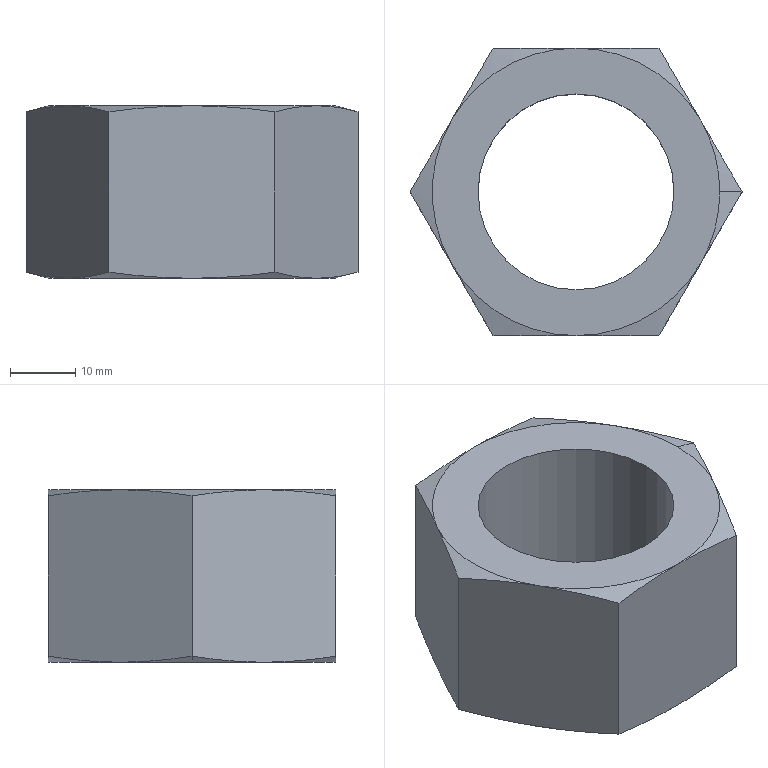Part | SolidWorks | features Cut 2, Chamfer 1, Extrusion 1 | 1 solid | 24 faces | box 50.85 x 44.037 x 26.4 mm | volume 25591 mm3 | cone 14 | plane 8 | cylinder 2 | commonest cylinder face diameters 30 x2
STEP:
#1=CARTESIAN_POINT('',(19.069,11.009,26.4));
#2=VERTEX_POINT('',#1);
#3=CARTESIAN_POINT('',(22.019,0.,26.4));
#4=VERTEX_POINT('',#3);
#5=CARTESIAN_POINT('',(0.,0.,26.4));
#6=DIRECTION('',(0.,0.,-1.));
#7=DIRECTION('',(-1.,0.,0.));
#8=AXIS2_PLACEMENT_3D('',#5,#6,#7);
#9=CIRCLE('',#8,22.019);
#10=EDGE_CURVE('',#2,#4,#9,.T.);
#11=ORIENTED_EDGE('',*,*,#10,.T.);
#12=CARTESIAN_POINT('',(25.425,0.,25.487));
#13=VERTEX_POINT('',#12);
#14=CARTESIAN_POINT('',(22.019,0.,26.4));
#15=DIRECTION('',(0.9659,0.,-0.2588));
#16=VECTOR('',#15,1000.);
#17=LINE('',#14,#16);
#18=EDGE_CURVE('',#4,#13,#17,.T.);
#19=ORIENTED_EDGE('',*,*,#18,.T.);
#20=CARTESIAN_POINT('',(25.425,0.,25.487));
#21=CARTESIAN_POINT('',(24.366,1.835,25.771));
#22=CARTESIAN_POINT('',(23.306,3.67,26.002));
#23=CARTESIAN_POINT('',(21.188,7.34,26.317));
#24=CARTESIAN_POINT('',(20.128,9.174,26.4));
#25=CARTESIAN_POINT('',(19.069,11.009,26.4));
#26=B_SPLINE_CURVE_WITH_KNOTS('',3,(#20,#21,#22,#23,#24,#25),.UNSPECIFIED.,.F.,.F.,(4,2,4),(0.000000231,0.006356,0.01271),.UNSPECIFIED.);
#27=EDGE_CURVE('',#13,#2,#26,.T.);
#28=ORIENTED_EDGE('',*,*,#27,.T.);
#29=EDGE_LOOP('',(#11,#19,#28));
#30=FACE_OUTER_BOUND('',#29,.T.);
#31=CARTESIAN_POINT('',(0.,0.,26.4));
#32=DIRECTION('',(0.,0.,-1.));
#33=DIRECTION('',(1.,0.,0.));
#34=AXIS2_PLACEMENT_3D('',#31,#32,#33);
#35=CONICAL_SURFACE('',#34,22.019,1.309);
#36=ADVANCED_FACE('',(#30),#35,.T.);
#37=CARTESIAN_POINT('',(-22.019,0.,0.));
#38=VERTEX_POINT('',#37);
#39=CARTESIAN_POINT('',(-19.069,11.009,0.));
#40=VERTEX_POINT('',#39);
#41=CARTESIAN_POINT('',(0.,0.,0.));
#42=DIRECTION('',(0.,0.,-1.));
#43=DIRECTION('',(-1.,0.,0.));
#44=AXIS2_PLACEMENT_3D('',#41,#42,#43);
#45=CIRCLE('',#44,22.019);
#46=EDGE_CURVE('',#38,#40,#45,.T.);
#47=ORIENTED_EDGE('',*,*,#46,.F.);
#48=CARTESIAN_POINT('',(-25.425,0.,0.9127));
#49=VERTEX_POINT('',#48);
#50=CARTESIAN_POINT('',(-22.019,0.,0.));
#51=DIRECTION('',(-0.9659,0.,0.2588));
#52=VECTOR('',#51,1000.);
#53=LINE('',#50,#52);
#54=EDGE_CURVE('',#38,#49,#53,.T.);
#55=ORIENTED_EDGE('',*,*,#54,.T.);
#56=CARTESIAN_POINT('',(-25.425,0.,0.9127));
#57=CARTESIAN_POINT('',(-24.366,1.835,0.6289));
#58=CARTESIAN_POINT('',(-23.306,3.67,0.3984));
#59=CARTESIAN_POINT('',(-21.187,7.34,0.08345));
#60=CARTESIAN_POINT('',(-20.128,9.174,0.));
#61=CARTESIAN_POINT('',(-19.069,11.009,0.));
#62=B_SPLINE_CURVE_WITH_KNOTS('',3,(#56,#57,#58,#59,#60,#61),.UNSPECIFIED.,.F.,.F.,(4,2,4),(0.000000231,0.006356,0.01271),.UNSPECIFIED.);
#63=EDGE_CURVE('',#49,#40,#62,.T.);
#64=ORIENTED_EDGE('',*,*,#63,.T.);
#65=EDGE_LOOP('',(#47,#55,#64));
#66=FACE_OUTER_BOUND('',#65,.T.);
#67=CARTESIAN_POINT('',(0.,0.,0.));
#68=DIRECTION('',(0.,0.,1.));
#69=DIRECTION('',(-1.,0.,0.));
#70=AXIS2_PLACEMENT_3D('',#67,#68,#69);
#71=CONICAL_SURFACE('',#70,22.019,1.309);
#72=ADVANCED_FACE('',(#66),#71,.T.);
#73=CARTESIAN_POINT('',(-15.,0.,26.4));
#74=VERTEX_POINT('',#73);
#75=CARTESIAN_POINT('',(15.,0.,26.4));
#76=VERTEX_POINT('',#75);
#77=CARTESIAN_POINT('',(0.,0.,26.4));
#78=DIRECTION('',(0.,0.,1.));
#79=DIRECTION('',(1.,0.,0.));
#80=AXIS2_PLACEMENT_3D('',#77,#78,#79);
#81=CIRCLE('',#80,15.);
#82=EDGE_CURVE('',#74,#76,#81,.T.);
#83=ORIENTED_EDGE('',*,*,#82,.T.);
#84=CARTESIAN_POINT('',(15.,0.,0.));
#85=VERTEX_POINT('',#84);
#86=CARTESIAN_POINT('',(15.,0.,26.4));
#87=DIRECTION('',(0.,0.,-1.));
#88=VECTOR('',#87,1000.);
#89=LINE('',#86,#88);
#90=EDGE_CURVE('',#76,#85,#89,.T.);
#91=ORIENTED_EDGE('',*,*,#90,.T.);
#92=CARTESIAN_POINT('',(-15.,0.,0.));
#93=VERTEX_POINT('',#92);
#94=CARTESIAN_POINT('',(0.,0.,0.));
#95=DIRECTION('',(0.,0.,1.));
#96=DIRECTION('',(1.,0.,0.));
#97=AXIS2_PLACEMENT_3D('',#94,#95,#96);
#98=CIRCLE('',#97,15.);
#99=EDGE_CURVE('',#93,#85,#98,.T.);
#100=ORIENTED_EDGE('',*,*,#99,.F.);
#101=CARTESIAN_POINT('',(-15.,0.,26.4));
#102=DIRECTION('',(0.,0.,-1.));
#103=VECTOR('',#102,1000.);
#104=LINE('',#101,#103);
#105=EDGE_CURVE('',#74,#93,#104,.T.);
#106=ORIENTED_EDGE('',*,*,#105,.F.);
#107=EDGE_LOOP('',(#83,#91,#100,#106));
#108=FACE_OUTER_BOUND('',#107,.T.);
#109=CARTESIAN_POINT('',(0.,0.,26.4));
#110=DIRECTION('',(0.,0.,-1.));
#111=DIRECTION('',(-1.,0.,0.));
#112=AXIS2_PLACEMENT_3D('',#109,#110,#111);
#113=CYLINDRICAL_SURFACE('',#112,15.);
#114=ADVANCED_FACE('',(#108),#113,.F.);
#115=ORIENTED_EDGE('',*,*,#27,.F.);
#116=CARTESIAN_POINT('',(25.425,0.,0.9127));
#117=VERTEX_POINT('',#116);
#118=CARTESIAN_POINT('',(25.425,0.,26.4));
#119=DIRECTION('',(0.,0.,-1.));
#120=VECTOR('',#119,1000.);
#121=LINE('',#118,#120);
#122=EDGE_CURVE('',#13,#117,#121,.T.);
#123=ORIENTED_EDGE('',*,*,#122,.T.);
#124=CARTESIAN_POINT('',(19.069,11.009,0.));
#125=VERTEX_POINT('',#124);
#126=CARTESIAN_POINT('',(19.069,11.009,0.));
#127=CARTESIAN_POINT('',(20.128,9.174,0.));
#128=CARTESIAN_POINT('',(21.188,7.34,0.08345));
#129=CARTESIAN_POINT('',(23.306,3.67,0.3984));
#130=CARTESIAN_POINT('',(24.366,1.835,0.6289));
#131=CARTESIAN_POINT('',(25.425,0.,0.9127));
#132=B_SPLINE_CURVE_WITH_KNOTS('',3,(#126,#127,#128,#129,#130,#131),.UNSPECIFIED.,.F.,.F.,(4,2,4),(0.01271,0.01907,0.02543),.UNSPECIFIED.);
#133=EDGE_CURVE('',#125,#117,#132,.T.);
#134=ORIENTED_EDGE('',*,*,#133,.F.);
#135=CARTESIAN_POINT('',(12.713,22.019,0.9127));
#136=VERTEX_POINT('',#135);
#137=CARTESIAN_POINT('',(12.713,22.019,0.9127));
#138=CARTESIAN_POINT('',(13.772,20.184,0.6289));
#139=CARTESIAN_POINT('',(14.831,18.349,0.3984));
#140=CARTESIAN_POINT('',(16.95,14.679,0.08345));
#141=CARTESIAN_POINT('',(18.009,12.844,0.));
#142=CARTESIAN_POINT('',(19.069,11.009,0.));
#143=B_SPLINE_CURVE_WITH_KNOTS('',3,(#137,#138,#139,#140,#141,#142),.UNSPECIFIED.,.F.,.F.,(4,2,4),(0.000000231,0.006356,0.01271),.UNSPECIFIED.);
#144=EDGE_CURVE('',#136,#125,#143,.T.);
#145=ORIENTED_EDGE('',*,*,#144,.F.);
#146=CARTESIAN_POINT('',(12.713,22.019,25.487));
#147=VERTEX_POINT('',#146);
#148=CARTESIAN_POINT('',(12.713,22.019,26.4));
#149=DIRECTION('',(0.,0.,-1.));
#150=VECTOR('',#149,1000.);
#151=LINE('',#148,#150);
#152=EDGE_CURVE('',#147,#136,#151,.T.);
#153=ORIENTED_EDGE('',*,*,#152,.F.);
#154=CARTESIAN_POINT('',(19.069,11.009,26.4));
#155=CARTESIAN_POINT('',(18.009,12.844,26.4));
#156=CARTESIAN_POINT('',(16.95,14.679,26.317));
#157=CARTESIAN_POINT('',(14.831,18.349,26.002));
#158=CARTESIAN_POINT('',(13.772,20.184,25.771));
#159=CARTESIAN_POINT('',(12.713,22.019,25.487));
#160=B_SPLINE_CURVE_WITH_KNOTS('',3,(#154,#155,#156,#157,#158,#159),.UNSPECIFIED.,.F.,.F.,(4,2,4),(0.01271,0.01907,0.02543),.UNSPECIFIED.);
#161=EDGE_CURVE('',#2,#147,#160,.T.);
#162=ORIENTED_EDGE('',*,*,#161,.F.);
#163=EDGE_LOOP('',(#115,#123,#134,#145,#153,#162));
#164=FACE_OUTER_BOUND('',#163,.T.);
#165=CARTESIAN_POINT('',(25.425,0.,26.4));
#166=DIRECTION('',(-0.866,-0.5,0.));
#167=DIRECTION('',(0.5,-0.866,0.));
#168=AXIS2_PLACEMENT_3D('',#165,#166,#167);
#169=PLANE('',#168);
#170=ADVANCED_FACE('',(#164),#169,.F.);
#171=CARTESIAN_POINT('',(0.,22.019,26.4));
#172=VERTEX_POINT('',#171);
#173=CARTESIAN_POINT('',(12.713,22.019,25.487));
#174=CARTESIAN_POINT('',(10.597,22.019,25.771));
#175=CARTESIAN_POINT('',(8.481,22.019,26.001));
#176=CARTESIAN_POINT('',(4.243,22.019,26.316));
#177=CARTESIAN_POINT('',(2.123,22.019,26.4));
#178=CARTESIAN_POINT('',(0.,22.019,26.4));
#179=B_SPLINE_CURVE_WITH_KNOTS('',3,(#173,#174,#175,#176,#177,#178),.UNSPECIFIED.,.F.,.F.,(4,2,4),(0.06895,0.07535,0.08174),.UNSPECIFIED.);
#180=EDGE_CURVE('',#147,#172,#179,.T.);
#181=ORIENTED_EDGE('',*,*,#180,.F.);
#182=ORIENTED_EDGE('',*,*,#152,.T.);
#183=CARTESIAN_POINT('',(0.,22.019,0.));
#184=VERTEX_POINT('',#183);
#185=CARTESIAN_POINT('',(0.,22.019,0.));
#186=CARTESIAN_POINT('',(2.123,22.019,0.));
#187=CARTESIAN_POINT('',(4.243,22.019,0.08376));
#188=CARTESIAN_POINT('',(8.481,22.019,0.3989));
#189=CARTESIAN_POINT('',(10.597,22.019,0.6293));
#190=CARTESIAN_POINT('',(12.713,22.019,0.9127));
#191=B_SPLINE_CURVE_WITH_KNOTS('',3,(#185,#186,#187,#188,#189,#190),.UNSPECIFIED.,.F.,.F.,(4,2,4),(0.03447,0.04087,0.04728),.UNSPECIFIED.);
#192=EDGE_CURVE('',#184,#136,#191,.T.);
#193=ORIENTED_EDGE('',*,*,#192,.F.);
#194=CARTESIAN_POINT('',(-12.712,22.019,0.9127));
#195=VERTEX_POINT('',#194);
#196=CARTESIAN_POINT('',(-12.712,22.019,0.9127));
#197=CARTESIAN_POINT('',(-10.6,22.019,0.6297));
#198=CARTESIAN_POINT('',(-8.474,22.019,0.3983));
#199=CARTESIAN_POINT('',(-4.234,22.019,0.08324));
#200=CARTESIAN_POINT('',(-2.116,22.019,0.));
#201=CARTESIAN_POINT('',(0.,22.019,0.));
#202=B_SPLINE_CURVE_WITH_KNOTS('',3,(#196,#197,#198,#199,#200,#201),.UNSPECIFIED.,.F.,.F.,(4,2,4),(0.02169,0.02808,0.03447),.UNSPECIFIED.);
#203=EDGE_CURVE('',#195,#184,#202,.T.);
#204=ORIENTED_EDGE('',*,*,#203,.F.);
#205=CARTESIAN_POINT('',(-12.712,22.019,25.487));
#206=VERTEX_POINT('',#205);
#207=CARTESIAN_POINT('',(-12.712,22.019,26.4));
#208=DIRECTION('',(0.,0.,-1.));
#209=VECTOR('',#208,1000.);
#210=LINE('',#207,#209);
#211=EDGE_CURVE('',#206,#195,#210,.T.);
#212=ORIENTED_EDGE('',*,*,#211,.F.);
#213=CARTESIAN_POINT('',(0.,22.019,26.4));
#214=CARTESIAN_POINT('',(-2.116,22.019,26.4));
#215=CARTESIAN_POINT('',(-4.234,22.019,26.317));
#216=CARTESIAN_POINT('',(-8.474,22.019,26.002));
#217=CARTESIAN_POINT('',(-10.6,22.019,25.77));
#218=CARTESIAN_POINT('',(-12.712,22.019,25.487));
#219=B_SPLINE_CURVE_WITH_KNOTS('',3,(#213,#214,#215,#216,#217,#218),.UNSPECIFIED.,.F.,.F.,(4,2,4),(0.08174,0.08811,0.09449),.UNSPECIFIED.);
#220=EDGE_CURVE('',#172,#206,#219,.T.);
#221=ORIENTED_EDGE('',*,*,#220,.F.);
#222=EDGE_LOOP('',(#181,#182,#193,#204,#212,#221));
#223=FACE_OUTER_BOUND('',#222,.T.);
#224=CARTESIAN_POINT('',(12.713,22.019,26.4));
#225=DIRECTION('',(0.,-1.,0.));
#226=DIRECTION('',(1.,0.,0.));
#227=AXIS2_PLACEMENT_3D('',#224,#225,#226);
#228=PLANE('',#227);
#229=ADVANCED_FACE('',(#223),#228,.F.);
#230=CARTESIAN_POINT('',(-19.069,11.009,26.4));
#231=VERTEX_POINT('',#230);
#232=CARTESIAN_POINT('',(-12.712,22.019,25.487));
#233=CARTESIAN_POINT('',(-13.772,20.184,25.771));
#234=CARTESIAN_POINT('',(-14.831,18.349,26.002));
#235=CARTESIAN_POINT('',(-16.95,14.679,26.317));
#236=CARTESIAN_POINT('',(-18.009,12.844,26.4));
#237=CARTESIAN_POINT('',(-19.069,11.009,26.4));
#238=B_SPLINE_CURVE_WITH_KNOTS('',3,(#232,#233,#234,#235,#236,#237),.UNSPECIFIED.,.F.,.F.,(4,2,4),(0.000000231,0.006356,0.01271),.UNSPECIFIED.);
#239=EDGE_CURVE('',#206,#231,#238,.T.);
#240=ORIENTED_EDGE('',*,*,#239,.F.);
#241=ORIENTED_EDGE('',*,*,#211,.T.);
#242=CARTESIAN_POINT('',(-19.069,11.009,0.));
#243=CARTESIAN_POINT('',(-18.009,12.844,0.));
#244=CARTESIAN_POINT('',(-16.95,14.679,0.08345));
#245=CARTESIAN_POINT('',(-14.831,18.349,0.3984));
#246=CARTESIAN_POINT('',(-13.772,20.184,0.6289));
#247=CARTESIAN_POINT('',(-12.712,22.019,0.9127));
#248=B_SPLINE_CURVE_WITH_KNOTS('',3,(#242,#243,#244,#245,#246,#247),.UNSPECIFIED.,.F.,.F.,(4,2,4),(0.01271,0.01907,0.02543),.UNSPECIFIED.);
#249=EDGE_CURVE('',#40,#195,#248,.T.);
#250=ORIENTED_EDGE('',*,*,#249,.F.);
#251=ORIENTED_EDGE('',*,*,#63,.F.);
#252=CARTESIAN_POINT('',(-25.425,0.,25.487));
#253=VERTEX_POINT('',#252);
#254=CARTESIAN_POINT('',(-25.425,0.,26.4));
#255=DIRECTION('',(0.,0.,-1.));
#256=VECTOR('',#255,1000.);
#257=LINE('',#254,#256);
#258=EDGE_CURVE('',#253,#49,#257,.T.);
#259=ORIENTED_EDGE('',*,*,#258,.F.);
#260=CARTESIAN_POINT('',(-19.069,11.009,26.4));
#261=CARTESIAN_POINT('',(-20.128,9.174,26.4));
#262=CARTESIAN_POINT('',(-21.187,7.34,26.317));
#263=CARTESIAN_POINT('',(-23.306,3.67,26.002));
#264=CARTESIAN_POINT('',(-24.366,1.835,25.771));
#265=CARTESIAN_POINT('',(-25.425,0.,25.487));
#266=B_SPLINE_CURVE_WITH_KNOTS('',3,(#260,#261,#262,#263,#264,#265),.UNSPECIFIED.,.F.,.F.,(4,2,4),(0.01271,0.01907,0.02543),.UNSPECIFIED.);
#267=EDGE_CURVE('',#231,#253,#266,.T.);
#268=ORIENTED_EDGE('',*,*,#267,.F.);
#269=EDGE_LOOP('',(#240,#241,#250,#251,#259,#268));
#270=FACE_OUTER_BOUND('',#269,.T.);
#271=CARTESIAN_POINT('',(-12.712,22.019,26.4));
#272=DIRECTION('',(0.866,-0.5,0.));
#273=DIRECTION('',(0.5,0.866,0.));
#274=AXIS2_PLACEMENT_3D('',#271,#272,#273);
#275=PLANE('',#274);
#276=ADVANCED_FACE('',(#270),#275,.F.);
#277=CARTESIAN_POINT('',(-19.069,-11.009,26.4));
#278=VERTEX_POINT('',#277);
#279=CARTESIAN_POINT('',(-25.425,0.,25.487));
#280=CARTESIAN_POINT('',(-24.366,-1.835,25.771));
#281=CARTESIAN_POINT('',(-23.306,-3.67,26.002));
#282=CARTESIAN_POINT('',(-21.187,-7.34,26.317));
#283=CARTESIAN_POINT('',(-20.128,-9.174,26.4));
#284=CARTESIAN_POINT('',(-19.069,-11.009,26.4));
#285=B_SPLINE_CURVE_WITH_KNOTS('',3,(#279,#280,#281,#282,#283,#284),.UNSPECIFIED.,.F.,.F.,(4,2,4),(0.000000231,0.006356,0.01271),.UNSPECIFIED.);
#286=EDGE_CURVE('',#253,#278,#285,.T.);
#287=ORIENTED_EDGE('',*,*,#286,.F.);
#288=ORIENTED_EDGE('',*,*,#258,.T.);
#289=CARTESIAN_POINT('',(-19.069,-11.009,0.));
#290=VERTEX_POINT('',#289);
#291=CARTESIAN_POINT('',(-19.069,-11.009,0.));
#292=CARTESIAN_POINT('',(-20.128,-9.174,0.));
#293=CARTESIAN_POINT('',(-21.188,-7.34,0.08345));
#294=CARTESIAN_POINT('',(-23.306,-3.67,0.3984));
#295=CARTESIAN_POINT('',(-24.366,-1.835,0.6289));
#296=CARTESIAN_POINT('',(-25.425,0.,0.9127));
#297=B_SPLINE_CURVE_WITH_KNOTS('',3,(#291,#292,#293,#294,#295,#296),.UNSPECIFIED.,.F.,.F.,(4,2,4),(0.01271,0.01907,0.02543),.UNSPECIFIED.);
#298=EDGE_CURVE('',#290,#49,#297,.T.);
#299=ORIENTED_EDGE('',*,*,#298,.F.);
#300=CARTESIAN_POINT('',(-12.713,-22.019,0.9127));
#301=VERTEX_POINT('',#300);
#302=CARTESIAN_POINT('',(-12.713,-22.019,0.9127));
#303=CARTESIAN_POINT('',(-13.772,-20.184,0.6289));
#304=CARTESIAN_POINT('',(-14.831,-18.349,0.3984));
#305=CARTESIAN_POINT('',(-16.95,-14.679,0.08345));
#306=CARTESIAN_POINT('',(-18.009,-12.844,0.));
#307=CARTESIAN_POINT('',(-19.069,-11.009,0.));
#308=B_SPLINE_CURVE_WITH_KNOTS('',3,(#302,#303,#304,#305,#306,#307),.UNSPECIFIED.,.F.,.F.,(4,2,4),(0.000000231,0.006356,0.01271),.UNSPECIFIED.);
#309=EDGE_CURVE('',#301,#290,#308,.T.);
#310=ORIENTED_EDGE('',*,*,#309,.F.);
#311=CARTESIAN_POINT('',(-12.713,-22.019,25.487));
#312=VERTEX_POINT('',#311);
#313=CARTESIAN_POINT('',(-12.712,-22.019,26.4));
#314=DIRECTION('',(0.,0.,-1.));
#315=VECTOR('',#314,1000.);
#316=LINE('',#313,#315);
#317=EDGE_CURVE('',#312,#301,#316,.T.);
#318=ORIENTED_EDGE('',*,*,#317,.F.);
#319=CARTESIAN_POINT('',(-19.069,-11.009,26.4));
#320=CARTESIAN_POINT('',(-18.009,-12.844,26.4));
#321=CARTESIAN_POINT('',(-16.95,-14.679,26.317));
#322=CARTESIAN_POINT('',(-14.831,-18.349,26.002));
#323=CARTESIAN_POINT('',(-13.772,-20.184,25.771));
#324=CARTESIAN_POINT('',(-12.713,-22.019,25.487));
#325=B_SPLINE_CURVE_WITH_KNOTS('',3,(#319,#320,#321,#322,#323,#324),.UNSPECIFIED.,.F.,.F.,(4,2,4),(0.01271,0.01907,0.02543),.UNSPECIFIED.);
#326=EDGE_CURVE('',#278,#312,#325,.T.);
#327=ORIENTED_EDGE('',*,*,#326,.F.);
#328=EDGE_LOOP('',(#287,#288,#299,#310,#318,#327));
#329=FACE_OUTER_BOUND('',#328,.T.);
#330=CARTESIAN_POINT('',(-25.425,0.,26.4));
#331=DIRECTION('',(0.866,0.5,0.));
#332=DIRECTION('',(-0.5,0.866,0.));
#333=AXIS2_PLACEMENT_3D('',#330,#331,#332);
#334=PLANE('',#333);
#335=ADVANCED_FACE('',(#329),#334,.F.);
#336=CARTESIAN_POINT('',(0.,-22.019,26.4));
#337=VERTEX_POINT('',#336);
#338=CARTESIAN_POINT('',(-12.713,-22.019,25.487));
#339=CARTESIAN_POINT('',(-10.6,-22.019,25.77));
#340=CARTESIAN_POINT('',(-8.474,-22.019,26.002));
#341=CARTESIAN_POINT('',(-4.234,-22.019,26.317));
#342=CARTESIAN_POINT('',(-2.116,-22.019,26.4));
#343=CARTESIAN_POINT('',(0.,-22.019,26.4));
#344=B_SPLINE_CURVE_WITH_KNOTS('',3,(#338,#339,#340,#341,#342,#343),.UNSPECIFIED.,.F.,.F.,(4,2,4),(0.02169,0.02808,0.03447),.UNSPECIFIED.);
#345=EDGE_CURVE('',#312,#337,#344,.T.);
#346=ORIENTED_EDGE('',*,*,#345,.F.);
#347=ORIENTED_EDGE('',*,*,#317,.T.);
#348=CARTESIAN_POINT('',(0.,-22.019,0.));
#349=VERTEX_POINT('',#348);
#350=CARTESIAN_POINT('',(0.,-22.019,0.));
#351=CARTESIAN_POINT('',(-2.116,-22.019,0.));
#352=CARTESIAN_POINT('',(-4.234,-22.019,0.08324));
#353=CARTESIAN_POINT('',(-8.474,-22.019,0.3983));
#354=CARTESIAN_POINT('',(-10.6,-22.019,0.6297));
#355=CARTESIAN_POINT('',(-12.713,-22.019,0.9127));
#356=B_SPLINE_CURVE_WITH_KNOTS('',3,(#350,#351,#352,#353,#354,#355),.UNSPECIFIED.,.F.,.F.,(4,2,4),(0.08174,0.08811,0.09449),.UNSPECIFIED.);
#357=EDGE_CURVE('',#349,#301,#356,.T.);
#358=ORIENTED_EDGE('',*,*,#357,.F.);
#359=CARTESIAN_POINT('',(12.713,-22.019,0.9127));
#360=VERTEX_POINT('',#359);
#361=CARTESIAN_POINT('',(12.713,-22.019,0.9127));
#362=CARTESIAN_POINT('',(10.597,-22.019,0.6293));
#363=CARTESIAN_POINT('',(8.481,-22.019,0.3989));
#364=CARTESIAN_POINT('',(4.243,-22.019,0.08376));
#365=CARTESIAN_POINT('',(2.123,-22.019,0.));
#366=CARTESIAN_POINT('',(0.,-22.019,0.));
#367=B_SPLINE_CURVE_WITH_KNOTS('',3,(#361,#362,#363,#364,#365,#366),.UNSPECIFIED.,.F.,.F.,(4,2,4),(0.06895,0.07535,0.08174),.UNSPECIFIED.);
#368=EDGE_CURVE('',#360,#349,#367,.T.);
#369=ORIENTED_EDGE('',*,*,#368,.F.);
#370=CARTESIAN_POINT('',(12.713,-22.019,25.487));
#371=VERTEX_POINT('',#370);
#372=CARTESIAN_POINT('',(12.713,-22.019,26.4));
#373=DIRECTION('',(0.,0.,-1.));
#374=VECTOR('',#373,1000.);
#375=LINE('',#372,#374);
#376=EDGE_CURVE('',#371,#360,#375,.T.);
#377=ORIENTED_EDGE('',*,*,#376,.F.);
#378=CARTESIAN_POINT('',(0.,-22.019,26.4));
#379=CARTESIAN_POINT('',(2.123,-22.019,26.4));
#380=CARTESIAN_POINT('',(4.243,-22.019,26.316));
#381=CARTESIAN_POINT('',(8.481,-22.019,26.001));
#382=CARTESIAN_POINT('',(10.597,-22.019,25.771));
#383=CARTESIAN_POINT('',(12.713,-22.019,25.487));
#384=B_SPLINE_CURVE_WITH_KNOTS('',3,(#378,#379,#380,#381,#382,#383),.UNSPECIFIED.,.F.,.F.,(4,2,4),(0.03447,0.04087,0.04728),.UNSPECIFIED.);
#385=EDGE_CURVE('',#337,#371,#384,.T.);
#386=ORIENTED_EDGE('',*,*,#385,.F.);
#387=EDGE_LOOP('',(#346,#347,#358,#369,#377,#386));
#388=FACE_OUTER_BOUND('',#387,.T.);
#389=CARTESIAN_POINT('',(-12.712,-22.019,26.4));
#390=DIRECTION('',(0.,1.,0.));
#391=DIRECTION('',(-1.,0.,0.));
#392=AXIS2_PLACEMENT_3D('',#389,#390,#391);
#393=PLANE('',#392);
#394=ADVANCED_FACE('',(#388),#393,.F.);
#395=CARTESIAN_POINT('',(19.069,-11.009,26.4));
#396=VERTEX_POINT('',#395);
#397=CARTESIAN_POINT('',(12.713,-22.019,25.487));
#398=CARTESIAN_POINT('',(13.772,-20.184,25.771));
#399=CARTESIAN_POINT('',(14.831,-18.349,26.002));
#400=CARTESIAN_POINT('',(16.95,-14.679,26.317));
#401=CARTESIAN_POINT('',(18.009,-12.844,26.4));
#402=CARTESIAN_POINT('',(19.069,-11.009,26.4));
#403=B_SPLINE_CURVE_WITH_KNOTS('',3,(#397,#398,#399,#400,#401,#402),.UNSPECIFIED.,.F.,.F.,(4,2,4),(0.000000231,0.006356,0.01271),.UNSPECIFIED.);
#404=EDGE_CURVE('',#371,#396,#403,.T.);
#405=ORIENTED_EDGE('',*,*,#404,.F.);
#406=ORIENTED_EDGE('',*,*,#376,.T.);
#407=CARTESIAN_POINT('',(19.069,-11.009,0.));
#408=VERTEX_POINT('',#407);
#409=CARTESIAN_POINT('',(19.069,-11.009,0.));
#410=CARTESIAN_POINT('',(18.009,-12.844,0.));
#411=CARTESIAN_POINT('',(16.95,-14.679,0.08345));
#412=CARTESIAN_POINT('',(14.831,-18.349,0.3984));
#413=CARTESIAN_POINT('',(13.772,-20.184,0.6289));
#414=CARTESIAN_POINT('',(12.713,-22.019,0.9127));
#415=B_SPLINE_CURVE_WITH_KNOTS('',3,(#409,#410,#411,#412,#413,#414),.UNSPECIFIED.,.F.,.F.,(4,2,4),(0.01271,0.01907,0.02543),.UNSPECIFIED.);
#416=EDGE_CURVE('',#408,#360,#415,.T.);
#417=ORIENTED_EDGE('',*,*,#416,.F.);
#418=CARTESIAN_POINT('',(25.425,0.,0.9127));
#419=CARTESIAN_POINT('',(24.366,-1.835,0.6289));
#420=CARTESIAN_POINT('',(23.306,-3.67,0.3984));
#421=CARTESIAN_POINT('',(21.188,-7.34,0.08345));
#422=CARTESIAN_POINT('',(20.128,-9.174,0.));
#423=CARTESIAN_POINT('',(19.069,-11.009,0.));
#424=B_SPLINE_CURVE_WITH_KNOTS('',3,(#418,#419,#420,#421,#422,#423),.UNSPECIFIED.,.F.,.F.,(4,2,4),(0.000000231,0.006356,0.01271),.UNSPECIFIED.);
#425=EDGE_CURVE('',#117,#408,#424,.T.);
#426=ORIENTED_EDGE('',*,*,#425,.F.);
#427=ORIENTED_EDGE('',*,*,#122,.F.);
#428=CARTESIAN_POINT('',(19.069,-11.009,26.4));
#429=CARTESIAN_POINT('',(20.128,-9.174,26.4));
#430=CARTESIAN_POINT('',(21.188,-7.34,26.317));
#431=CARTESIAN_POINT('',(23.306,-3.67,26.002));
#432=CARTESIAN_POINT('',(24.366,-1.835,25.771));
#433=CARTESIAN_POINT('',(25.425,0.,25.487));
#434=B_SPLINE_CURVE_WITH_KNOTS('',3,(#428,#429,#430,#431,#432,#433),.UNSPECIFIED.,.F.,.F.,(4,2,4),(0.01271,0.01907,0.02543),.UNSPECIFIED.);
#435=EDGE_CURVE('',#396,#13,#434,.T.);
#436=ORIENTED_EDGE('',*,*,#435,.F.);
#437=EDGE_LOOP('',(#405,#406,#417,#426,#427,#436));
#438=FACE_OUTER_BOUND('',#437,.T.);
#439=CARTESIAN_POINT('',(12.713,-22.019,26.4));
#440=DIRECTION('',(-0.866,0.5,0.));
#441=DIRECTION('',(-0.5,-0.866,0.));
#442=AXIS2_PLACEMENT_3D('',#439,#440,#441);
#443=PLANE('',#442);
#444=ADVANCED_FACE('',(#438),#443,.F.);
#445=ORIENTED_EDGE('',*,*,#82,.F.);
#446=CARTESIAN_POINT('',(0.,0.,26.4));
#447=DIRECTION('',(0.,0.,1.));
#448=DIRECTION('',(1.,0.,0.));
#449=AXIS2_PLACEMENT_3D('',#446,#447,#448);
#450=CIRCLE('',#449,15.);
#451=EDGE_CURVE('',#76,#74,#450,.T.);
#452=ORIENTED_EDGE('',*,*,#451,.F.);
#453=EDGE_LOOP('',(#445,#452));
#454=FACE_BOUND('',#453,.T.);
#455=CARTESIAN_POINT('',(0.,0.,26.4));
#456=DIRECTION('',(0.,0.,-1.));
#457=DIRECTION('',(-1.,0.,0.));
#458=AXIS2_PLACEMENT_3D('',#455,#456,#457);
#459=CIRCLE('',#458,22.019);
#460=EDGE_CURVE('',#231,#172,#459,.T.);
#461=ORIENTED_EDGE('',*,*,#460,.F.);
#462=CARTESIAN_POINT('',(0.,0.,26.4));
#463=DIRECTION('',(0.,0.,-1.));
#464=DIRECTION('',(-1.,0.,0.));
#465=AXIS2_PLACEMENT_3D('',#462,#463,#464);
#466=CIRCLE('',#465,22.019);
#467=EDGE_CURVE('',#278,#231,#466,.T.);
#468=ORIENTED_EDGE('',*,*,#467,.F.);
#469=CARTESIAN_POINT('',(0.,0.,26.4));
#470=DIRECTION('',(0.,0.,-1.));
#471=DIRECTION('',(-1.,0.,0.));
#472=AXIS2_PLACEMENT_3D('',#469,#470,#471);
#473=CIRCLE('',#472,22.019);
#474=EDGE_CURVE('',#337,#278,#473,.T.);
#475=ORIENTED_EDGE('',*,*,#474,.F.);
#476=CARTESIAN_POINT('',(0.,0.,26.4));
#477=DIRECTION('',(0.,0.,-1.));
#478=DIRECTION('',(-1.,0.,0.));
#479=AXIS2_PLACEMENT_3D('',#476,#477,#478);
#480=CIRCLE('',#479,22.019);
#481=EDGE_CURVE('',#396,#337,#480,.T.);
#482=ORIENTED_EDGE('',*,*,#481,.F.);
#483=CARTESIAN_POINT('',(0.,0.,26.4));
#484=DIRECTION('',(0.,0.,-1.));
#485=DIRECTION('',(-1.,0.,0.));
#486=AXIS2_PLACEMENT_3D('',#483,#484,#485);
#487=CIRCLE('',#486,22.019);
#488=EDGE_CURVE('',#4,#396,#487,.T.);
#489=ORIENTED_EDGE('',*,*,#488,.F.);
#490=ORIENTED_EDGE('',*,*,#10,.F.);
#491=CARTESIAN_POINT('',(0.,0.,26.4));
#492=DIRECTION('',(0.,0.,1.));
#493=DIRECTION('',(1.,0.,0.));
#494=AXIS2_PLACEMENT_3D('',#491,#492,#493);
#495=CIRCLE('',#494,22.019);
#496=EDGE_CURVE('',#2,#172,#495,.T.);
#497=ORIENTED_EDGE('',*,*,#496,.T.);
#498=EDGE_LOOP('',(#461,#468,#475,#482,#489,#490,#497));
#499=FACE_OUTER_BOUND('',#498,.T.);
#500=CARTESIAN_POINT('',(38.137,-22.019,26.4));
#501=DIRECTION('',(0.,0.,-1.));
#502=DIRECTION('',(-1.,0.,0.));
#503=AXIS2_PLACEMENT_3D('',#500,#501,#502);
#504=PLANE('',#503);
#505=ADVANCED_FACE('',(#454,#499),#504,.F.);
#506=ORIENTED_EDGE('',*,*,#99,.T.);
#507=CARTESIAN_POINT('',(0.,0.,0.));
#508=DIRECTION('',(0.,0.,1.));
#509=DIRECTION('',(1.,0.,0.));
#510=AXIS2_PLACEMENT_3D('',#507,#508,#509);
#511=CIRCLE('',#510,15.);
#512=EDGE_CURVE('',#85,#93,#511,.T.);
#513=ORIENTED_EDGE('',*,*,#512,.T.);
#514=EDGE_LOOP('',(#506,#513));
#515=FACE_BOUND('',#514,.T.);
#516=CARTESIAN_POINT('',(0.,0.,0.));
#517=DIRECTION('',(0.,0.,-1.));
#518=DIRECTION('',(-1.,0.,0.));
#519=AXIS2_PLACEMENT_3D('',#516,#517,#518);
#520=CIRCLE('',#519,22.019);
#521=EDGE_CURVE('',#290,#38,#520,.T.);
#522=ORIENTED_EDGE('',*,*,#521,.T.);
#523=ORIENTED_EDGE('',*,*,#46,.T.);
#524=CARTESIAN_POINT('',(0.,0.,0.));
#525=DIRECTION('',(0.,0.,-1.));
#526=DIRECTION('',(-1.,0.,0.));
#527=AXIS2_PLACEMENT_3D('',#524,#525,#526);
#528=CIRCLE('',#527,22.019);
#529=EDGE_CURVE('',#40,#184,#528,.T.);
#530=ORIENTED_EDGE('',*,*,#529,.T.);
#531=CARTESIAN_POINT('',(0.,0.,0.));
#532=DIRECTION('',(0.,0.,-1.));
#533=DIRECTION('',(-1.,0.,0.));
#534=AXIS2_PLACEMENT_3D('',#531,#532,#533);
#535=CIRCLE('',#534,22.019);
#536=EDGE_CURVE('',#184,#125,#535,.T.);
#537=ORIENTED_EDGE('',*,*,#536,.T.);
#538=CARTESIAN_POINT('',(0.,0.,0.));
#539=DIRECTION('',(0.,0.,-1.));
#540=DIRECTION('',(-1.,0.,0.));
#541=AXIS2_PLACEMENT_3D('',#538,#539,#540);
#542=CIRCLE('',#541,22.019);
#543=EDGE_CURVE('',#125,#408,#542,.T.);
#544=ORIENTED_EDGE('',*,*,#543,.T.);
#545=CARTESIAN_POINT('',(0.,0.,0.));
#546=DIRECTION('',(0.,0.,-1.));
#547=DIRECTION('',(-1.,0.,0.));
#548=AXIS2_PLACEMENT_3D('',#545,#546,#547);
#549=CIRCLE('',#548,22.019);
#550=EDGE_CURVE('',#408,#349,#549,.T.);
#551=ORIENTED_EDGE('',*,*,#550,.T.);
#552=CARTESIAN_POINT('',(0.,0.,0.));
#553=DIRECTION('',(0.,0.,-1.));
#554=DIRECTION('',(-1.,0.,0.));
#555=AXIS2_PLACEMENT_3D('',#552,#553,#554);
#556=CIRCLE('',#555,22.019);
#557=EDGE_CURVE('',#349,#290,#556,.T.);
#558=ORIENTED_EDGE('',*,*,#557,.T.);
#559=EDGE_LOOP('',(#522,#523,#530,#537,#544,#551,#558));
#560=FACE_OUTER_BOUND('',#559,.T.);
#561=CARTESIAN_POINT('',(38.137,-22.019,0.));
#562=DIRECTION('',(0.,0.,-1.));
#563=DIRECTION('',(-1.,0.,0.));
#564=AXIS2_PLACEMENT_3D('',#561,#562,#563);
#565=PLANE('',#564);
#566=ADVANCED_FACE('',(#515,#560),#565,.T.);
#567=ORIENTED_EDGE('',*,*,#90,.F.);
#568=ORIENTED_EDGE('',*,*,#451,.T.);
#569=ORIENTED_EDGE('',*,*,#105,.T.);
#570=ORIENTED_EDGE('',*,*,#512,.F.);
#571=EDGE_LOOP('',(#567,#568,#569,#570));
#572=FACE_OUTER_BOUND('',#571,.T.);
#573=CARTESIAN_POINT('',(0.,0.,26.4));
#574=DIRECTION('',(0.,0.,-1.));
#575=DIRECTION('',(-1.,0.,0.));
#576=AXIS2_PLACEMENT_3D('',#573,#574,#575);
#577=CYLINDRICAL_SURFACE('',#576,15.);
#578=ADVANCED_FACE('',(#572),#577,.F.);
#579=ORIENTED_EDGE('',*,*,#368,.T.);
#580=ORIENTED_EDGE('',*,*,#550,.F.);
#581=ORIENTED_EDGE('',*,*,#416,.T.);
#582=EDGE_LOOP('',(#579,#580,#581));
#583=FACE_OUTER_BOUND('',#582,.T.);
#584=CARTESIAN_POINT('',(0.,0.,0.));
#585=DIRECTION('',(0.,0.,1.));
#586=DIRECTION('',(-1.,0.,0.));
#587=AXIS2_PLACEMENT_3D('',#584,#585,#586);
#588=CONICAL_SURFACE('',#587,22.019,1.309);
#589=ADVANCED_FACE('',(#583),#588,.T.);
#590=ORIENTED_EDGE('',*,*,#133,.T.);
#591=ORIENTED_EDGE('',*,*,#425,.T.);
#592=ORIENTED_EDGE('',*,*,#543,.F.);
#593=EDGE_LOOP('',(#590,#591,#592));
#594=FACE_OUTER_BOUND('',#593,.T.);
#595=CARTESIAN_POINT('',(0.,0.,0.));
#596=DIRECTION('',(0.,0.,1.));
#597=DIRECTION('',(-1.,0.,0.));
#598=AXIS2_PLACEMENT_3D('',#595,#596,#597);
#599=CONICAL_SURFACE('',#598,22.019,1.309);
#600=ADVANCED_FACE('',(#594),#599,.T.);
#601=ORIENTED_EDGE('',*,*,#309,.T.);
#602=ORIENTED_EDGE('',*,*,#557,.F.);
#603=ORIENTED_EDGE('',*,*,#357,.T.);
#604=EDGE_LOOP('',(#601,#602,#603));
#605=FACE_OUTER_BOUND('',#604,.T.);
#606=CARTESIAN_POINT('',(0.,0.,0.));
#607=DIRECTION('',(0.,0.,1.));
#608=DIRECTION('',(-1.,0.,0.));
#609=AXIS2_PLACEMENT_3D('',#606,#607,#608);
#610=CONICAL_SURFACE('',#609,22.019,1.309);
#611=ADVANCED_FACE('',(#605),#610,.T.);
#612=ORIENTED_EDGE('',*,*,#54,.F.);
#613=ORIENTED_EDGE('',*,*,#521,.F.);
#614=ORIENTED_EDGE('',*,*,#298,.T.);
#615=EDGE_LOOP('',(#612,#613,#614));
#616=FACE_OUTER_BOUND('',#615,.T.);
#617=CARTESIAN_POINT('',(0.,0.,0.));
#618=DIRECTION('',(0.,0.,1.));
#619=DIRECTION('',(-1.,0.,0.));
#620=AXIS2_PLACEMENT_3D('',#617,#618,#619);
#621=CONICAL_SURFACE('',#620,22.019,1.309);
#622=ADVANCED_FACE('',(#616),#621,.T.);
#623=ORIENTED_EDGE('',*,*,#249,.T.);
#624=ORIENTED_EDGE('',*,*,#203,.T.);
#625=ORIENTED_EDGE('',*,*,#529,.F.);
#626=EDGE_LOOP('',(#623,#624,#625));
#627=FACE_OUTER_BOUND('',#626,.T.);
#628=CARTESIAN_POINT('',(0.,0.,0.));
#629=DIRECTION('',(0.,0.,1.));
#630=DIRECTION('',(-1.,0.,0.));
#631=AXIS2_PLACEMENT_3D('',#628,#629,#630);
#632=CONICAL_SURFACE('',#631,22.019,1.309);
#633=ADVANCED_FACE('',(#627),#632,.T.);
#634=ORIENTED_EDGE('',*,*,#192,.T.);
#635=ORIENTED_EDGE('',*,*,#144,.T.);
#636=ORIENTED_EDGE('',*,*,#536,.F.);
#637=EDGE_LOOP('',(#634,#635,#636));
#638=FACE_OUTER_BOUND('',#637,.T.);
#639=CARTESIAN_POINT('',(0.,0.,0.));
#640=DIRECTION('',(0.,0.,1.));
#641=DIRECTION('',(-1.,0.,0.));
#642=AXIS2_PLACEMENT_3D('',#639,#640,#641);
#643=CONICAL_SURFACE('',#642,22.019,1.309);
#644=ADVANCED_FACE('',(#638),#643,.T.);
#645=ORIENTED_EDGE('',*,*,#267,.T.);
#646=ORIENTED_EDGE('',*,*,#286,.T.);
#647=ORIENTED_EDGE('',*,*,#467,.T.);
#648=EDGE_LOOP('',(#645,#646,#647));
#649=FACE_OUTER_BOUND('',#648,.T.);
#650=CARTESIAN_POINT('',(0.,0.,26.4));
#651=DIRECTION('',(0.,0.,-1.));
#652=DIRECTION('',(1.,0.,0.));
#653=AXIS2_PLACEMENT_3D('',#650,#651,#652);
#654=CONICAL_SURFACE('',#653,22.019,1.309);
#655=ADVANCED_FACE('',(#649),#654,.T.);
#656=ORIENTED_EDGE('',*,*,#326,.T.);
#657=ORIENTED_EDGE('',*,*,#345,.T.);
#658=ORIENTED_EDGE('',*,*,#474,.T.);
#659=EDGE_LOOP('',(#656,#657,#658));
#660=FACE_OUTER_BOUND('',#659,.T.);
#661=CARTESIAN_POINT('',(0.,0.,26.4));
#662=DIRECTION('',(0.,0.,-1.));
#663=DIRECTION('',(1.,0.,0.));
#664=AXIS2_PLACEMENT_3D('',#661,#662,#663);
#665=CONICAL_SURFACE('',#664,22.019,1.309);
#666=ADVANCED_FACE('',(#660),#665,.T.);
#667=ORIENTED_EDGE('',*,*,#385,.T.);
#668=ORIENTED_EDGE('',*,*,#404,.T.);
#669=ORIENTED_EDGE('',*,*,#481,.T.);
#670=EDGE_LOOP('',(#667,#668,#669));
#671=FACE_OUTER_BOUND('',#670,.T.);
#672=CARTESIAN_POINT('',(0.,0.,26.4));
#673=DIRECTION('',(0.,0.,-1.));
#674=DIRECTION('',(1.,0.,0.));
#675=AXIS2_PLACEMENT_3D('',#672,#673,#674);
#676=CONICAL_SURFACE('',#675,22.019,1.309);
#677=ADVANCED_FACE('',(#671),#676,.T.);
#678=ORIENTED_EDGE('',*,*,#18,.F.);
#679=ORIENTED_EDGE('',*,*,#488,.T.);
#680=ORIENTED_EDGE('',*,*,#435,.T.);
#681=EDGE_LOOP('',(#678,#679,#680));
#682=FACE_OUTER_BOUND('',#681,.T.);
#683=CARTESIAN_POINT('',(0.,0.,26.4));
#684=DIRECTION('',(0.,0.,-1.));
#685=DIRECTION('',(1.,0.,0.));
#686=AXIS2_PLACEMENT_3D('',#683,#684,#685);
#687=CONICAL_SURFACE('',#686,22.019,1.309);
#688=ADVANCED_FACE('',(#682),#687,.T.);
#689=ORIENTED_EDGE('',*,*,#161,.T.);
#690=ORIENTED_EDGE('',*,*,#180,.T.);
#691=ORIENTED_EDGE('',*,*,#496,.F.);
#692=EDGE_LOOP('',(#689,#690,#691));
#693=FACE_OUTER_BOUND('',#692,.T.);
#694=CARTESIAN_POINT('',(0.,0.,26.4));
#695=DIRECTION('',(0.,0.,-1.));
#696=DIRECTION('',(1.,0.,0.));
#697=AXIS2_PLACEMENT_3D('',#694,#695,#696);
#698=CONICAL_SURFACE('',#697,22.019,1.309);
#699=ADVANCED_FACE('',(#693),#698,.T.);
#700=ORIENTED_EDGE('',*,*,#220,.T.);
#701=ORIENTED_EDGE('',*,*,#239,.T.);
#702=ORIENTED_EDGE('',*,*,#460,.T.);
#703=EDGE_LOOP('',(#700,#701,#702));
#704=FACE_OUTER_BOUND('',#703,.T.);
#705=CARTESIAN_POINT('',(0.,0.,26.4));
#706=DIRECTION('',(0.,0.,-1.));
#707=DIRECTION('',(1.,0.,0.));
#708=AXIS2_PLACEMENT_3D('',#705,#706,#707);
#709=CONICAL_SURFACE('',#708,22.019,1.309);
#710=ADVANCED_FACE('',(#704),#709,.T.);
#711=CLOSED_SHELL('',(#36,#72,#114,#170,#229,#276,#335,#394,#444,#505,#566,#578,#589,#600,#611,#622,#633,#644,#655,#666,#677,#688,#699,#710));
#712=MANIFOLD_SOLID_BREP('',#711);
#713=CARTESIAN_POINT('',(0.,0.,0.));
#714=DIRECTION('',(0.,0.,1.));
#715=DIRECTION('',(1.,0.,0.));
#716=AXIS2_PLACEMENT_3D('',#713,#714,#715);
#717=(LENGTH_UNIT()NAMED_UNIT(*)SI_UNIT(.MILLI.,.METRE.));
#718=UNCERTAINTY_MEASURE_WITH_UNIT(LENGTH_MEASURE(0.00001),#717,'','');
#719=(NAMED_UNIT(*)PLANE_ANGLE_UNIT()SI_UNIT($,.RADIAN.));
#720=(NAMED_UNIT(*)SI_UNIT($,.STERADIAN.)SOLID_ANGLE_UNIT());
#721=(GEOMETRIC_REPRESENTATION_CONTEXT(3)GLOBAL_UNCERTAINTY_ASSIGNED_CONTEXT((#718))GLOBAL_UNIT_ASSIGNED_CONTEXT((#717,#719,#720))REPRESENTATION_CONTEXT('',''));
#722=ADVANCED_BREP_SHAPE_REPRESENTATION('',(#712,#716),#721);